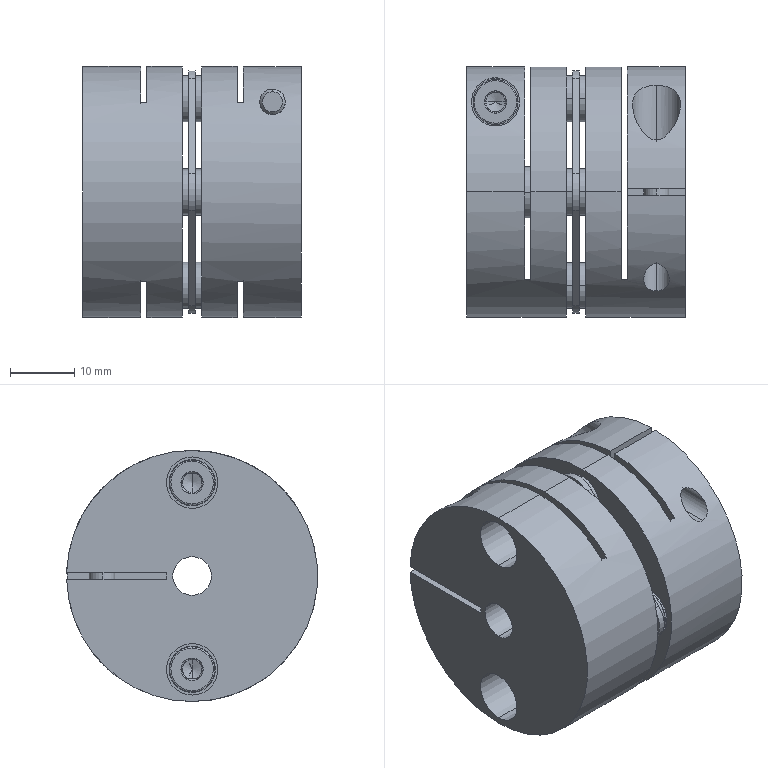Part | STEP file | SFC-035SA2-6B-12B_2_03 | 1 solid | 222 faces | box 34 x 39 x 39 mm | volume 30442 mm3 | plane 107 | cylinder 75 | cone 28 | spline 12 | commonest cylinder face diameters 8 x21 7.2 x16 7 x12 4 x8 39 x7 7.5 x4